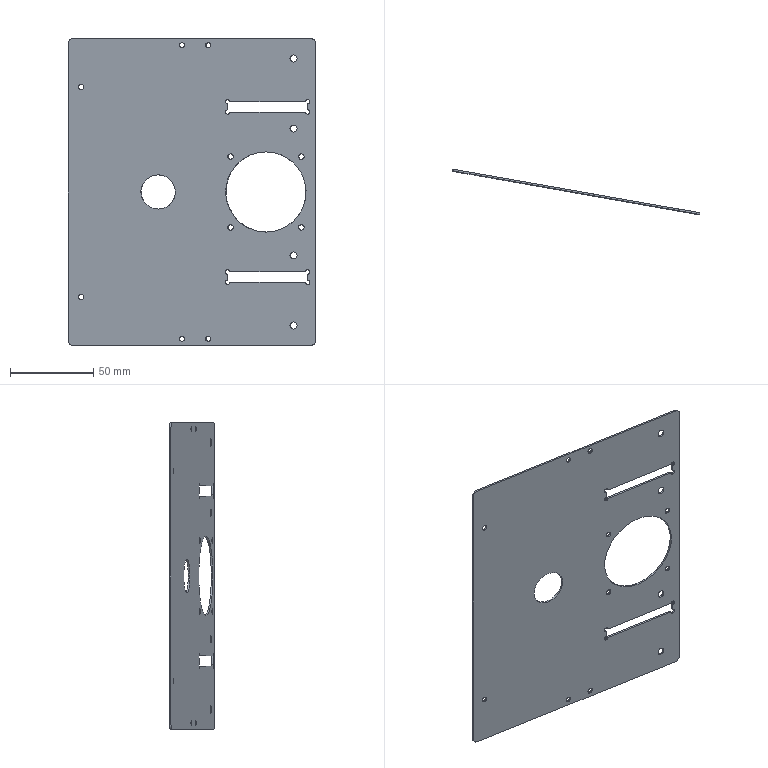Part | SolidWorks | features ICE 7, Fillet 3, Cut 1, Extrusion 1 | 1 solid | 82 faces | box 148.62 x 27.16 x 184 mm | volume 24771 mm3 | cylinder 54 | plane 14 | spline 14 | commonest cylinder face diameters 3.2 x24 2.5 x12 4.3 x8 6 x4 20.5 x3 48 x3